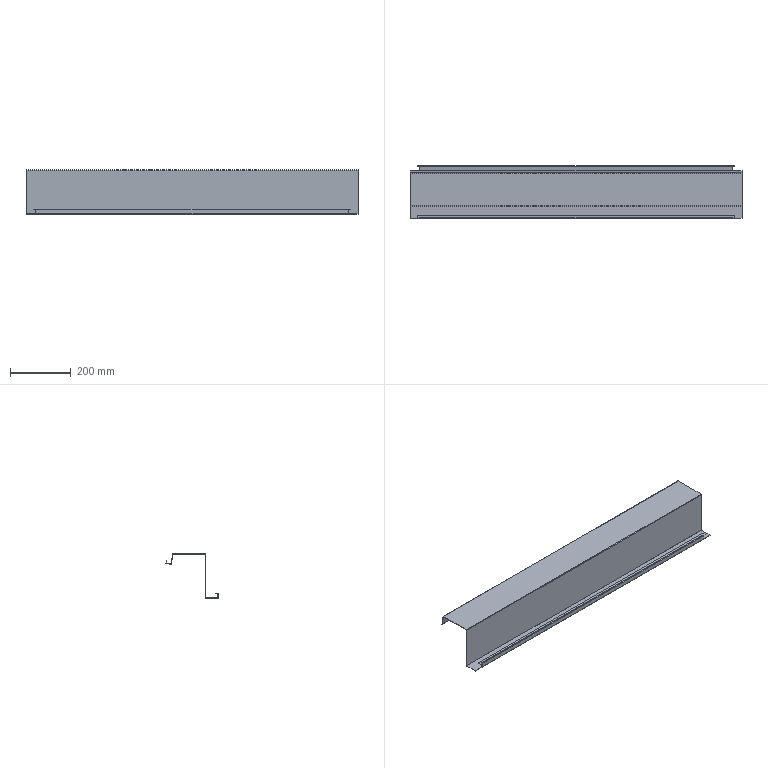Part | SolidWorks | features EdgeFlange 7, SMBaseFlange 3, FlatPattern 1, SheetMetal 1 | 1 solid | 94 faces | box 1097 x 172.327 x 146.5 mm | volume 612727 mm3 | plane 80 | cylinder 14 | commonest cylinder face diameters 0.2 x7 3.2 x7